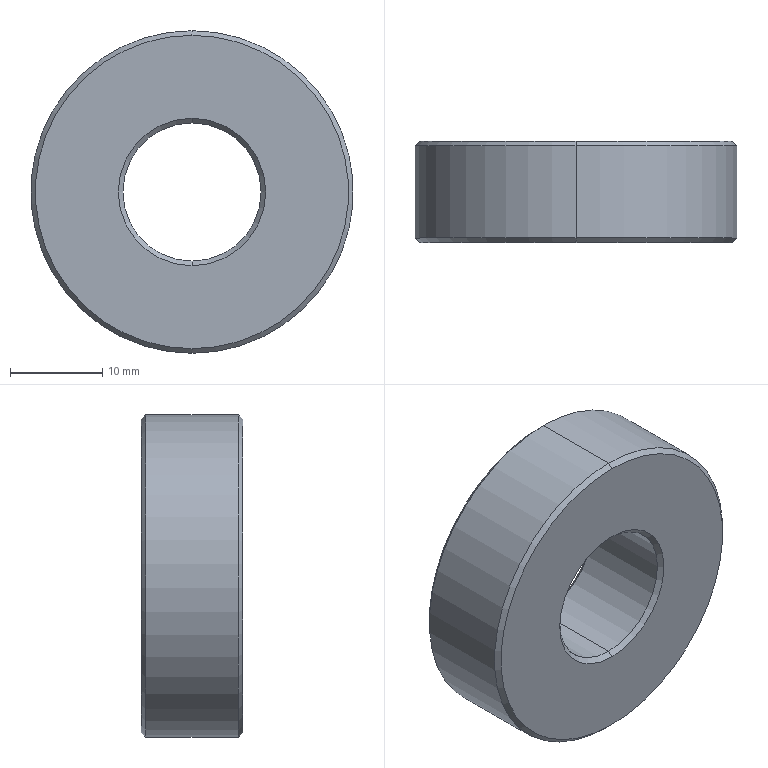Part | SolidWorks | features MirrorStock 1 | 1 solid | 14 faces | box 35 x 11 x 35 mm | volume 8600 mm3 | cone 8 | cylinder 4 | plane 2 | commonest cylinder face diameters 15 x2 35 x2
STEP:
#1=CARTESIAN_POINT('',(0.,10.5,-7.5));
#2=VERTEX_POINT('',#1);
#3=CARTESIAN_POINT('',(0.,10.5,7.5));
#4=VERTEX_POINT('',#3);
#5=CARTESIAN_POINT('',(0.,10.5,0.));
#6=DIRECTION('',(0.,-1.,0.));
#7=DIRECTION('',(0.,0.,-1.));
#8=AXIS2_PLACEMENT_3D('',#5,#6,#7);
#9=CIRCLE('',#8,7.5);
#10=EDGE_CURVE('',#2,#4,#9,.T.);
#11=ORIENTED_EDGE('',*,*,#10,.T.);
#12=CARTESIAN_POINT('',(0.,11.,8.));
#13=VERTEX_POINT('',#12);
#14=CARTESIAN_POINT('',(0.,10.5,7.5));
#15=DIRECTION('',(0.,0.7071,0.7071));
#16=VECTOR('',#15,1000.);
#17=LINE('',#14,#16);
#18=EDGE_CURVE('',#4,#13,#17,.T.);
#19=ORIENTED_EDGE('',*,*,#18,.T.);
#20=CARTESIAN_POINT('',(0.,11.,-8.));
#21=VERTEX_POINT('',#20);
#22=CARTESIAN_POINT('',(0.,11.,0.));
#23=DIRECTION('',(0.,1.,0.));
#24=DIRECTION('',(0.,0.,-1.));
#25=AXIS2_PLACEMENT_3D('',#22,#23,#24);
#26=CIRCLE('',#25,8.);
#27=EDGE_CURVE('',#13,#21,#26,.T.);
#28=ORIENTED_EDGE('',*,*,#27,.T.);
#29=CARTESIAN_POINT('',(0.,10.5,-7.5));
#30=DIRECTION('',(0.,0.7071,-0.7071));
#31=VECTOR('',#30,1000.);
#32=LINE('',#29,#31);
#33=EDGE_CURVE('',#2,#21,#32,.T.);
#34=ORIENTED_EDGE('',*,*,#33,.F.);
#35=EDGE_LOOP('',(#11,#19,#28,#34));
#36=FACE_OUTER_BOUND('',#35,.T.);
#37=CARTESIAN_POINT('',(0.,10.5,0.));
#38=DIRECTION('',(0.,1.,0.));
#39=DIRECTION('',(0.,0.,-1.));
#40=AXIS2_PLACEMENT_3D('',#37,#38,#39);
#41=CONICAL_SURFACE('',#40,7.5,0.7854);
#42=ADVANCED_FACE('',(#36),#41,.F.);
#43=CARTESIAN_POINT('',(0.,11.,17.));
#44=VERTEX_POINT('',#43);
#45=CARTESIAN_POINT('',(0.,11.,-17.));
#46=VERTEX_POINT('',#45);
#47=CARTESIAN_POINT('',(0.,11.,0.));
#48=DIRECTION('',(0.,-1.,0.));
#49=DIRECTION('',(0.,0.,-1.));
#50=AXIS2_PLACEMENT_3D('',#47,#48,#49);
#51=CIRCLE('',#50,17.);
#52=EDGE_CURVE('',#44,#46,#51,.T.);
#53=ORIENTED_EDGE('',*,*,#52,.T.);
#54=CARTESIAN_POINT('',(0.,10.5,-17.5));
#55=VERTEX_POINT('',#54);
#56=CARTESIAN_POINT('',(0.,11.,-17.));
#57=DIRECTION('',(0.,-0.7071,-0.7071));
#58=VECTOR('',#57,1000.);
#59=LINE('',#56,#58);
#60=EDGE_CURVE('',#46,#55,#59,.T.);
#61=ORIENTED_EDGE('',*,*,#60,.T.);
#62=CARTESIAN_POINT('',(0.,10.5,17.5));
#63=VERTEX_POINT('',#62);
#64=CARTESIAN_POINT('',(0.,10.5,0.));
#65=DIRECTION('',(0.,1.,0.));
#66=DIRECTION('',(0.,0.,-1.));
#67=AXIS2_PLACEMENT_3D('',#64,#65,#66);
#68=CIRCLE('',#67,17.5);
#69=EDGE_CURVE('',#55,#63,#68,.T.);
#70=ORIENTED_EDGE('',*,*,#69,.T.);
#71=CARTESIAN_POINT('',(0.,11.,17.));
#72=DIRECTION('',(0.,-0.7071,0.7071));
#73=VECTOR('',#72,1000.);
#74=LINE('',#71,#73);
#75=EDGE_CURVE('',#44,#63,#74,.T.);
#76=ORIENTED_EDGE('',*,*,#75,.F.);
#77=EDGE_LOOP('',(#53,#61,#70,#76));
#78=FACE_OUTER_BOUND('',#77,.T.);
#79=CARTESIAN_POINT('',(0.,11.,0.));
#80=DIRECTION('',(0.,-1.,0.));
#81=DIRECTION('',(0.,0.,1.));
#82=AXIS2_PLACEMENT_3D('',#79,#80,#81);
#83=CONICAL_SURFACE('',#82,17.,0.7854);
#84=ADVANCED_FACE('',(#78),#83,.T.);
#85=CARTESIAN_POINT('',(0.,0.,-17.));
#86=VERTEX_POINT('',#85);
#87=CARTESIAN_POINT('',(0.,0.,17.));
#88=VERTEX_POINT('',#87);
#89=CARTESIAN_POINT('',(0.,0.,0.));
#90=DIRECTION('',(0.,1.,0.));
#91=DIRECTION('',(0.,0.,-1.));
#92=AXIS2_PLACEMENT_3D('',#89,#90,#91);
#93=CIRCLE('',#92,17.);
#94=EDGE_CURVE('',#86,#88,#93,.T.);
#95=ORIENTED_EDGE('',*,*,#94,.T.);
#96=CARTESIAN_POINT('',(0.,0.5,17.5));
#97=VERTEX_POINT('',#96);
#98=CARTESIAN_POINT('',(0.,0.5,17.5));
#99=DIRECTION('',(0.,0.7071,0.7071));
#100=VECTOR('',#99,1000.);
#101=LINE('',#98,#100);
#102=EDGE_CURVE('',#88,#97,#101,.T.);
#103=ORIENTED_EDGE('',*,*,#102,.T.);
#104=CARTESIAN_POINT('',(0.,0.5,-17.5));
#105=VERTEX_POINT('',#104);
#106=CARTESIAN_POINT('',(0.,0.5,0.));
#107=DIRECTION('',(0.,-1.,0.));
#108=DIRECTION('',(0.,0.,-1.));
#109=AXIS2_PLACEMENT_3D('',#106,#107,#108);
#110=CIRCLE('',#109,17.5);
#111=EDGE_CURVE('',#97,#105,#110,.T.);
#112=ORIENTED_EDGE('',*,*,#111,.T.);
#113=CARTESIAN_POINT('',(0.,0.5,-17.5));
#114=DIRECTION('',(0.,0.7071,-0.7071));
#115=VECTOR('',#114,1000.);
#116=LINE('',#113,#115);
#117=EDGE_CURVE('',#86,#105,#116,.T.);
#118=ORIENTED_EDGE('',*,*,#117,.F.);
#119=EDGE_LOOP('',(#95,#103,#112,#118));
#120=FACE_OUTER_BOUND('',#119,.T.);
#121=CARTESIAN_POINT('',(0.,0.5,0.));
#122=DIRECTION('',(0.,1.,0.));
#123=DIRECTION('',(0.,0.,-1.));
#124=AXIS2_PLACEMENT_3D('',#121,#122,#123);
#125=CONICAL_SURFACE('',#124,17.5,0.7854);
#126=ADVANCED_FACE('',(#120),#125,.T.);
#127=CARTESIAN_POINT('',(0.,0.5,7.5));
#128=VERTEX_POINT('',#127);
#129=CARTESIAN_POINT('',(0.,0.5,-7.5));
#130=VERTEX_POINT('',#129);
#131=CARTESIAN_POINT('',(0.,0.5,0.));
#132=DIRECTION('',(0.,1.,0.));
#133=DIRECTION('',(0.,0.,-1.));
#134=AXIS2_PLACEMENT_3D('',#131,#132,#133);
#135=CIRCLE('',#134,7.5);
#136=EDGE_CURVE('',#128,#130,#135,.T.);
#137=ORIENTED_EDGE('',*,*,#136,.T.);
#138=CARTESIAN_POINT('',(0.,0.,-8.));
#139=VERTEX_POINT('',#138);
#140=CARTESIAN_POINT('',(0.,0.,-8.));
#141=DIRECTION('',(0.,-0.7071,-0.7071));
#142=VECTOR('',#141,1000.);
#143=LINE('',#140,#142);
#144=EDGE_CURVE('',#130,#139,#143,.T.);
#145=ORIENTED_EDGE('',*,*,#144,.T.);
#146=CARTESIAN_POINT('',(0.,0.,8.));
#147=VERTEX_POINT('',#146);
#148=CARTESIAN_POINT('',(0.,0.,0.));
#149=DIRECTION('',(0.,-1.,0.));
#150=DIRECTION('',(0.,0.,-1.));
#151=AXIS2_PLACEMENT_3D('',#148,#149,#150);
#152=CIRCLE('',#151,8.);
#153=EDGE_CURVE('',#139,#147,#152,.T.);
#154=ORIENTED_EDGE('',*,*,#153,.T.);
#155=CARTESIAN_POINT('',(0.,0.,8.));
#156=DIRECTION('',(0.,-0.7071,0.7071));
#157=VECTOR('',#156,1000.);
#158=LINE('',#155,#157);
#159=EDGE_CURVE('',#128,#147,#158,.T.);
#160=ORIENTED_EDGE('',*,*,#159,.F.);
#161=EDGE_LOOP('',(#137,#145,#154,#160));
#162=FACE_OUTER_BOUND('',#161,.T.);
#163=CARTESIAN_POINT('',(0.,0.,0.));
#164=DIRECTION('',(0.,-1.,0.));
#165=DIRECTION('',(0.,0.,1.));
#166=AXIS2_PLACEMENT_3D('',#163,#164,#165);
#167=CONICAL_SURFACE('',#166,8.,0.7854);
#168=ADVANCED_FACE('',(#162),#167,.F.);
#169=ORIENTED_EDGE('',*,*,#10,.F.);
#170=CARTESIAN_POINT('',(0.,11.,-7.5));
#171=DIRECTION('',(0.,-1.,0.));
#172=VECTOR('',#171,1000.);
#173=LINE('',#170,#172);
#174=EDGE_CURVE('',#2,#130,#173,.T.);
#175=ORIENTED_EDGE('',*,*,#174,.T.);
#176=ORIENTED_EDGE('',*,*,#136,.F.);
#177=CARTESIAN_POINT('',(0.,11.,7.5));
#178=DIRECTION('',(0.,-1.,0.));
#179=VECTOR('',#178,1000.);
#180=LINE('',#177,#179);
#181=EDGE_CURVE('',#4,#128,#180,.T.);
#182=ORIENTED_EDGE('',*,*,#181,.F.);
#183=EDGE_LOOP('',(#169,#175,#176,#182));
#184=FACE_OUTER_BOUND('',#183,.T.);
#185=CARTESIAN_POINT('',(0.,11.,0.));
#186=DIRECTION('',(0.,-1.,0.));
#187=DIRECTION('',(0.,0.,1.));
#188=AXIS2_PLACEMENT_3D('',#185,#186,#187);
#189=CYLINDRICAL_SURFACE('',#188,7.5);
#190=ADVANCED_FACE('',(#184),#189,.F.);
#191=ORIENTED_EDGE('',*,*,#69,.F.);
#192=CARTESIAN_POINT('',(0.,11.,-17.5));
#193=DIRECTION('',(0.,-1.,0.));
#194=VECTOR('',#193,1000.);
#195=LINE('',#192,#194);
#196=EDGE_CURVE('',#55,#105,#195,.T.);
#197=ORIENTED_EDGE('',*,*,#196,.T.);
#198=ORIENTED_EDGE('',*,*,#111,.F.);
#199=CARTESIAN_POINT('',(0.,11.,17.5));
#200=DIRECTION('',(0.,-1.,0.));
#201=VECTOR('',#200,1000.);
#202=LINE('',#199,#201);
#203=EDGE_CURVE('',#63,#97,#202,.T.);
#204=ORIENTED_EDGE('',*,*,#203,.F.);
#205=EDGE_LOOP('',(#191,#197,#198,#204));
#206=FACE_OUTER_BOUND('',#205,.T.);
#207=CARTESIAN_POINT('',(0.,11.,0.));
#208=DIRECTION('',(0.,-1.,0.));
#209=DIRECTION('',(0.,0.,1.));
#210=AXIS2_PLACEMENT_3D('',#207,#208,#209);
#211=CYLINDRICAL_SURFACE('',#210,17.5);
#212=ADVANCED_FACE('',(#206),#211,.T.);
#213=ORIENTED_EDGE('',*,*,#52,.F.);
#214=CARTESIAN_POINT('',(0.,11.,0.));
#215=DIRECTION('',(0.,-1.,0.));
#216=DIRECTION('',(0.,0.,-1.));
#217=AXIS2_PLACEMENT_3D('',#214,#215,#216);
#218=CIRCLE('',#217,17.);
#219=EDGE_CURVE('',#46,#44,#218,.T.);
#220=ORIENTED_EDGE('',*,*,#219,.F.);
#221=EDGE_LOOP('',(#213,#220));
#222=FACE_OUTER_BOUND('',#221,.T.);
#223=CARTESIAN_POINT('',(0.,11.,0.));
#224=DIRECTION('',(0.,1.,0.));
#225=DIRECTION('',(0.,0.,-1.));
#226=AXIS2_PLACEMENT_3D('',#223,#224,#225);
#227=CIRCLE('',#226,8.);
#228=EDGE_CURVE('',#21,#13,#227,.T.);
#229=ORIENTED_EDGE('',*,*,#228,.F.);
#230=ORIENTED_EDGE('',*,*,#27,.F.);
#231=EDGE_LOOP('',(#229,#230));
#232=FACE_BOUND('',#231,.T.);
#233=CARTESIAN_POINT('',(0.,11.,0.));
#234=DIRECTION('',(0.,1.,0.));
#235=DIRECTION('',(0.,0.,-1.));
#236=AXIS2_PLACEMENT_3D('',#233,#234,#235);
#237=PLANE('',#236);
#238=ADVANCED_FACE('',(#222,#232),#237,.T.);
#239=CARTESIAN_POINT('',(0.,0.,0.));
#240=DIRECTION('',(0.,-1.,0.));
#241=DIRECTION('',(0.,0.,-1.));
#242=AXIS2_PLACEMENT_3D('',#239,#240,#241);
#243=CIRCLE('',#242,8.);
#244=EDGE_CURVE('',#147,#139,#243,.T.);
#245=ORIENTED_EDGE('',*,*,#244,.F.);
#246=ORIENTED_EDGE('',*,*,#153,.F.);
#247=EDGE_LOOP('',(#245,#246));
#248=FACE_BOUND('',#247,.T.);
#249=ORIENTED_EDGE('',*,*,#94,.F.);
#250=CARTESIAN_POINT('',(0.,0.,0.));
#251=DIRECTION('',(0.,1.,0.));
#252=DIRECTION('',(0.,0.,-1.));
#253=AXIS2_PLACEMENT_3D('',#250,#251,#252);
#254=CIRCLE('',#253,17.);
#255=EDGE_CURVE('',#88,#86,#254,.T.);
#256=ORIENTED_EDGE('',*,*,#255,.F.);
#257=EDGE_LOOP('',(#249,#256));
#258=FACE_OUTER_BOUND('',#257,.T.);
#259=CARTESIAN_POINT('',(0.,0.,0.));
#260=DIRECTION('',(0.,1.,0.));
#261=DIRECTION('',(0.,0.,-1.));
#262=AXIS2_PLACEMENT_3D('',#259,#260,#261);
#263=PLANE('',#262);
#264=ADVANCED_FACE('',(#248,#258),#263,.F.);
#265=ORIENTED_EDGE('',*,*,#196,.F.);
#266=CARTESIAN_POINT('',(0.,10.5,0.));
#267=DIRECTION('',(0.,1.,0.));
#268=DIRECTION('',(0.,0.,-1.));
#269=AXIS2_PLACEMENT_3D('',#266,#267,#268);
#270=CIRCLE('',#269,17.5);
#271=EDGE_CURVE('',#63,#55,#270,.T.);
#272=ORIENTED_EDGE('',*,*,#271,.F.);
#273=ORIENTED_EDGE('',*,*,#203,.T.);
#274=CARTESIAN_POINT('',(0.,0.5,0.));
#275=DIRECTION('',(0.,-1.,0.));
#276=DIRECTION('',(0.,0.,-1.));
#277=AXIS2_PLACEMENT_3D('',#274,#275,#276);
#278=CIRCLE('',#277,17.5);
#279=EDGE_CURVE('',#105,#97,#278,.T.);
#280=ORIENTED_EDGE('',*,*,#279,.F.);
#281=EDGE_LOOP('',(#265,#272,#273,#280));
#282=FACE_OUTER_BOUND('',#281,.T.);
#283=CARTESIAN_POINT('',(0.,11.,0.));
#284=DIRECTION('',(0.,-1.,0.));
#285=DIRECTION('',(0.,0.,1.));
#286=AXIS2_PLACEMENT_3D('',#283,#284,#285);
#287=CYLINDRICAL_SURFACE('',#286,17.5);
#288=ADVANCED_FACE('',(#282),#287,.T.);
#289=ORIENTED_EDGE('',*,*,#174,.F.);
#290=CARTESIAN_POINT('',(0.,10.5,0.));
#291=DIRECTION('',(0.,-1.,0.));
#292=DIRECTION('',(0.,0.,-1.));
#293=AXIS2_PLACEMENT_3D('',#290,#291,#292);
#294=CIRCLE('',#293,7.5);
#295=EDGE_CURVE('',#4,#2,#294,.T.);
#296=ORIENTED_EDGE('',*,*,#295,.F.);
#297=ORIENTED_EDGE('',*,*,#181,.T.);
#298=CARTESIAN_POINT('',(0.,0.5,0.));
#299=DIRECTION('',(0.,1.,0.));
#300=DIRECTION('',(0.,0.,-1.));
#301=AXIS2_PLACEMENT_3D('',#298,#299,#300);
#302=CIRCLE('',#301,7.5);
#303=EDGE_CURVE('',#130,#128,#302,.T.);
#304=ORIENTED_EDGE('',*,*,#303,.F.);
#305=EDGE_LOOP('',(#289,#296,#297,#304));
#306=FACE_OUTER_BOUND('',#305,.T.);
#307=CARTESIAN_POINT('',(0.,11.,0.));
#308=DIRECTION('',(0.,-1.,0.));
#309=DIRECTION('',(0.,0.,1.));
#310=AXIS2_PLACEMENT_3D('',#307,#308,#309);
#311=CYLINDRICAL_SURFACE('',#310,7.5);
#312=ADVANCED_FACE('',(#306),#311,.F.);
#313=ORIENTED_EDGE('',*,*,#144,.F.);
#314=ORIENTED_EDGE('',*,*,#303,.T.);
#315=ORIENTED_EDGE('',*,*,#159,.T.);
#316=ORIENTED_EDGE('',*,*,#244,.T.);
#317=EDGE_LOOP('',(#313,#314,#315,#316));
#318=FACE_OUTER_BOUND('',#317,.T.);
#319=CARTESIAN_POINT('',(0.,0.,0.));
#320=DIRECTION('',(0.,-1.,0.));
#321=DIRECTION('',(0.,0.,1.));
#322=AXIS2_PLACEMENT_3D('',#319,#320,#321);
#323=CONICAL_SURFACE('',#322,8.,0.7854);
#324=ADVANCED_FACE('',(#318),#323,.F.);
#325=ORIENTED_EDGE('',*,*,#102,.F.);
#326=ORIENTED_EDGE('',*,*,#255,.T.);
#327=ORIENTED_EDGE('',*,*,#117,.T.);
#328=ORIENTED_EDGE('',*,*,#279,.T.);
#329=EDGE_LOOP('',(#325,#326,#327,#328));
#330=FACE_OUTER_BOUND('',#329,.T.);
#331=CARTESIAN_POINT('',(0.,0.5,0.));
#332=DIRECTION('',(0.,1.,0.));
#333=DIRECTION('',(0.,0.,-1.));
#334=AXIS2_PLACEMENT_3D('',#331,#332,#333);
#335=CONICAL_SURFACE('',#334,17.5,0.7854);
#336=ADVANCED_FACE('',(#330),#335,.T.);
#337=ORIENTED_EDGE('',*,*,#60,.F.);
#338=ORIENTED_EDGE('',*,*,#219,.T.);
#339=ORIENTED_EDGE('',*,*,#75,.T.);
#340=ORIENTED_EDGE('',*,*,#271,.T.);
#341=EDGE_LOOP('',(#337,#338,#339,#340));
#342=FACE_OUTER_BOUND('',#341,.T.);
#343=CARTESIAN_POINT('',(0.,11.,0.));
#344=DIRECTION('',(0.,-1.,0.));
#345=DIRECTION('',(0.,0.,1.));
#346=AXIS2_PLACEMENT_3D('',#343,#344,#345);
#347=CONICAL_SURFACE('',#346,17.,0.7854);
#348=ADVANCED_FACE('',(#342),#347,.T.);
#349=ORIENTED_EDGE('',*,*,#18,.F.);
#350=ORIENTED_EDGE('',*,*,#295,.T.);
#351=ORIENTED_EDGE('',*,*,#33,.T.);
#352=ORIENTED_EDGE('',*,*,#228,.T.);
#353=EDGE_LOOP('',(#349,#350,#351,#352));
#354=FACE_OUTER_BOUND('',#353,.T.);
#355=CARTESIAN_POINT('',(0.,10.5,0.));
#356=DIRECTION('',(0.,1.,0.));
#357=DIRECTION('',(0.,0.,-1.));
#358=AXIS2_PLACEMENT_3D('',#355,#356,#357);
#359=CONICAL_SURFACE('',#358,7.5,0.7854);
#360=ADVANCED_FACE('',(#354),#359,.F.);
#361=CLOSED_SHELL('',(#42,#84,#126,#168,#190,#212,#238,#264,#288,#312,#324,#336,#348,#360));
#362=MANIFOLD_SOLID_BREP('',#361);
#363=CARTESIAN_POINT('',(0.,0.,0.));
#364=DIRECTION('',(0.,0.,1.));
#365=DIRECTION('',(1.,0.,0.));
#366=AXIS2_PLACEMENT_3D('',#363,#364,#365);
#367=(LENGTH_UNIT()NAMED_UNIT(*)SI_UNIT(.MILLI.,.METRE.));
#368=UNCERTAINTY_MEASURE_WITH_UNIT(LENGTH_MEASURE(0.00001),#367,'','');
#369=(NAMED_UNIT(*)PLANE_ANGLE_UNIT()SI_UNIT($,.RADIAN.));
#370=(NAMED_UNIT(*)SI_UNIT($,.STERADIAN.)SOLID_ANGLE_UNIT());
#371=(GEOMETRIC_REPRESENTATION_CONTEXT(3)GLOBAL_UNCERTAINTY_ASSIGNED_CONTEXT((#368))GLOBAL_UNIT_ASSIGNED_CONTEXT((#367,#369,#370))REPRESENTATION_CONTEXT('',''));
#372=ADVANCED_BREP_SHAPE_REPRESENTATION('',(#362,#366),#371);